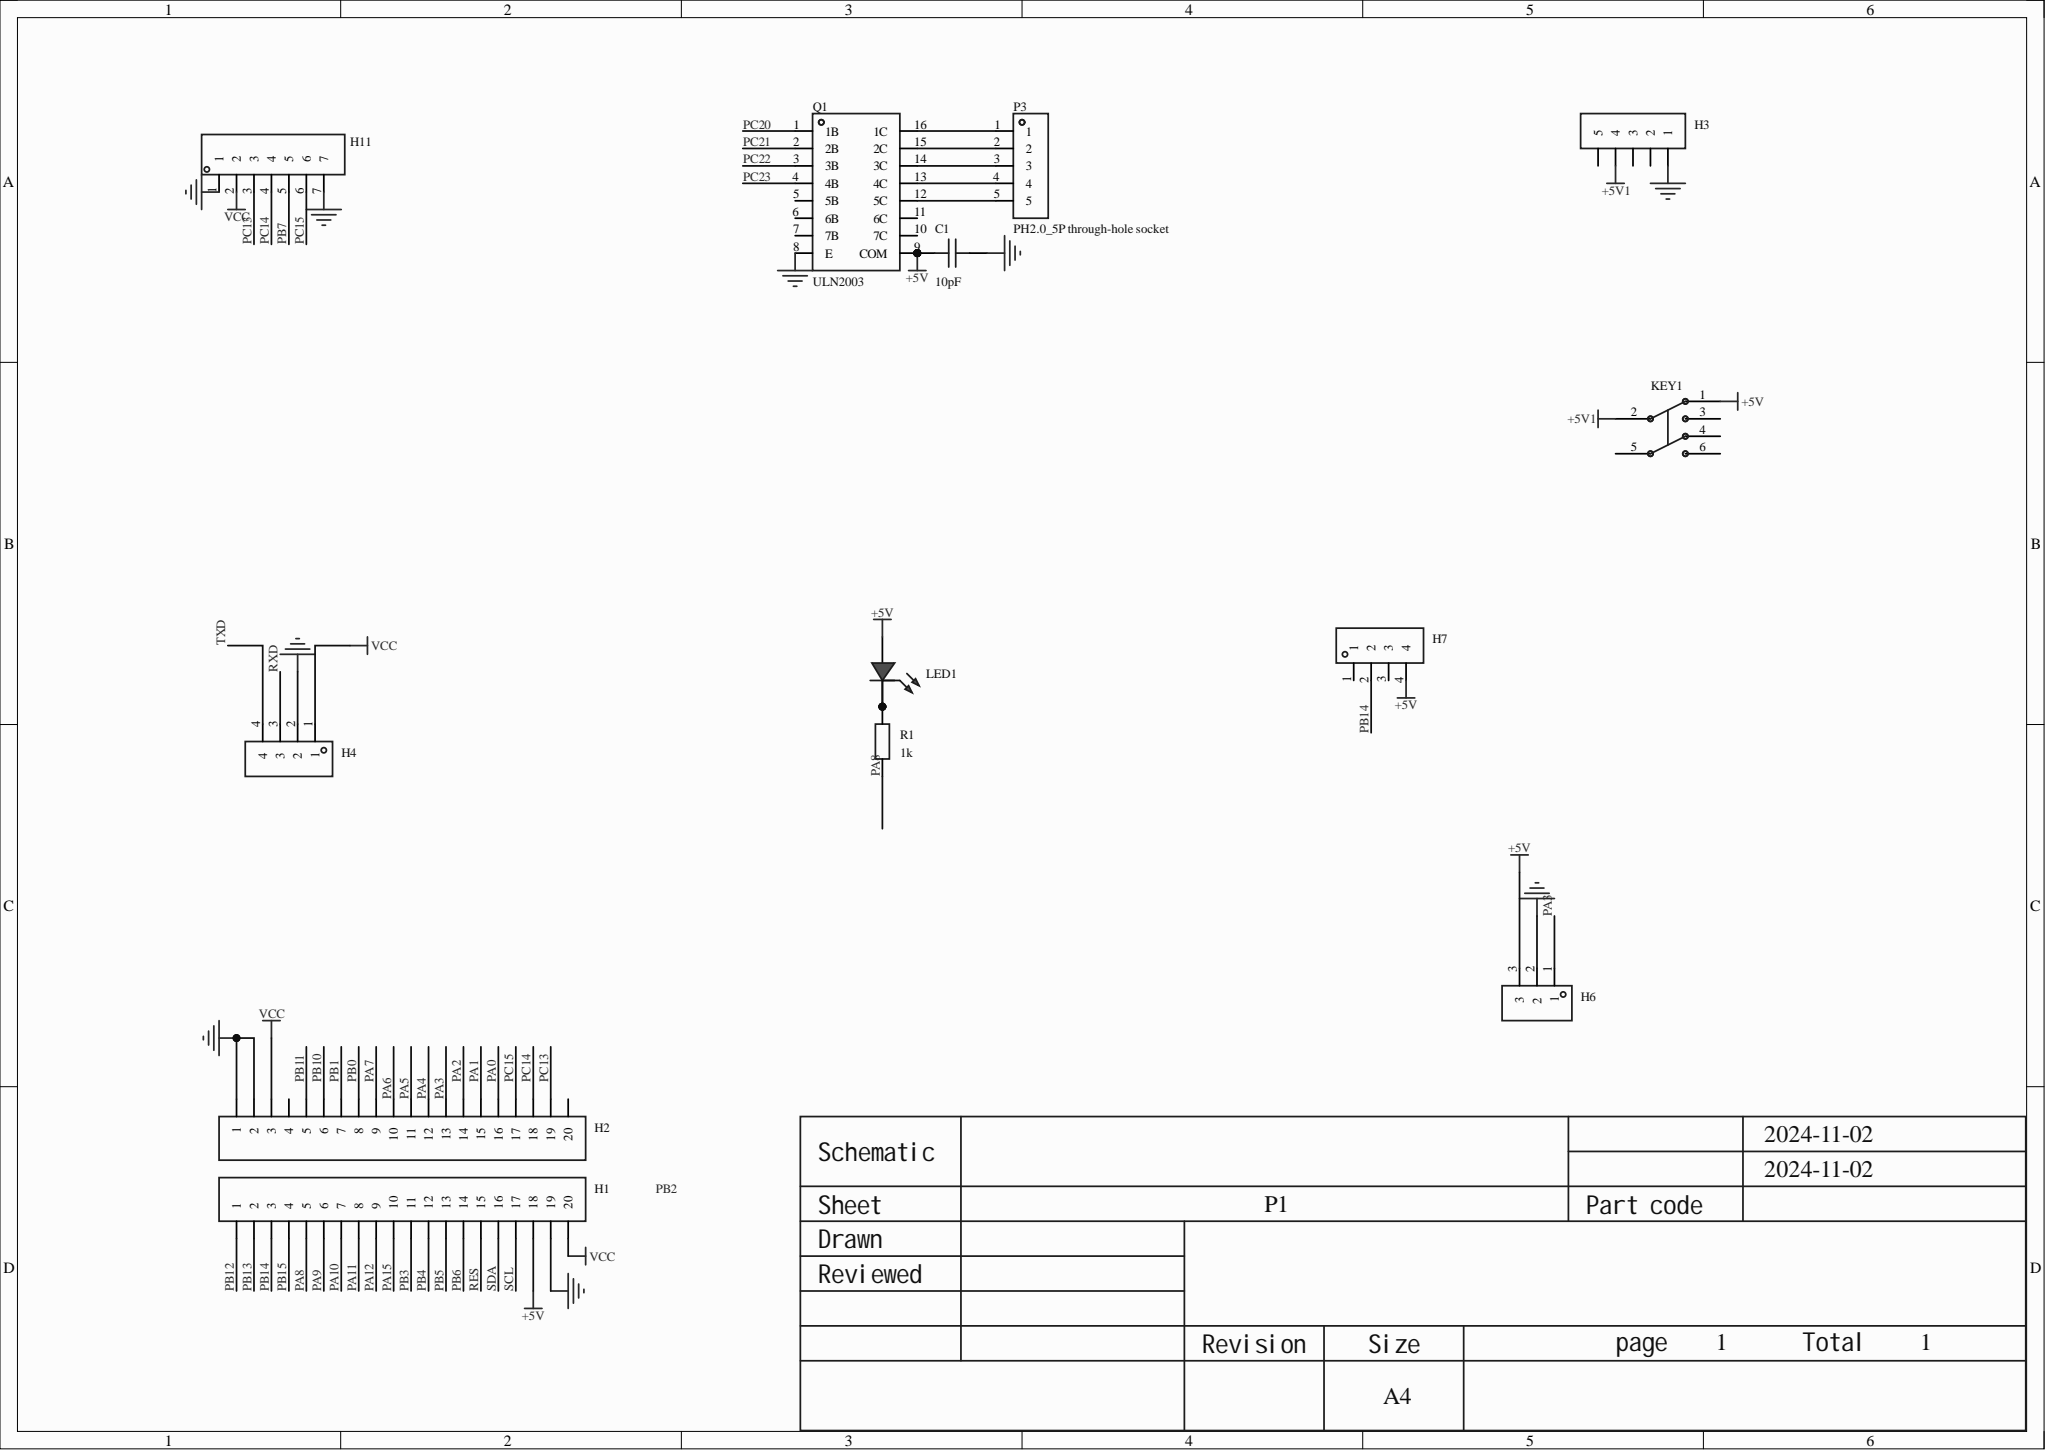Circuit board | Altium Designer | 13 parts | 16 nets
Bill of materials:
Comment,Description,Designator,Footprint,LibRef,Quantity
"10pF","容值:10pF;精度:±5%;额定电压:3kV;温度系数:SL;","C1","CAP-TH_L5.5-W6.0-P7.50-D0.6","CC45SL3FD100JYGNA","1"
"","","H1, H2","HDR-TH_20P-P2.54-V-F","HDR-F_2.54_1x20P","2"
"","","H3","HDR-TH_5P-P2.54-V-F","HDR-F_2.54_1x5P","1"
"","","H4, H7","HDR-TH_4P-P2.54-V-F","HDR-F_2.54_1x4P","2"
"","","H6","HDR-TH_3P-P2.54-V-F","HDR-F_2.54_1x3P","1"
"","","H11","HDR-TH_7P-P2.54-V-F","HDR-F_2.54_1x7P","1"
"Non-self-locking switch 8.5×8.5 silent","6脚，8.5×8.5","KEY1","SW-TH_6P-L8.5-W8.5-P2.54","无自锁开关 8.5×8.5 无声","1"
"","","LED1","LED_TH-_5mm","LED_TH-R_5mm","1"
"PH2.0_5P through-hole socket","","P3","CONN-TH_5P-P2.00-PH5A","PH2.0_5P直插插座","1"
"ULN2003","","Q1","DIP-16_L19.8-W6.5-P2.54-LS7.6-BL","ULN2003_C557872","1"
"1k","","R1","Res_1/4W","Res_AXIAL-1/4W","1"
Netlist (Protel format):
[
C1
CAP-TH_L5.5-W6.0-P7.50-D0.6
10pF



]
[
H1
HDR-TH_20P-P2.54-V-F




]
[
H2
HDR-TH_20P-P2.54-V-F




]
[
H3
HDR-TH_5P-P2.54-V-F




]
[
H4
HDR-TH_4P-P2.54-V-F




]
[
H6
HDR-TH_3P-P2.54-V-F




]
[
H7
HDR-TH_4P-P2.54-V-F




]
[
H11
HDR-TH_7P-P2.54-V-F




]
[
KEY1
SW-TH_6P-L8.5-W8.5-P2.54
Non-self-locking switch 8.5×8.5 silent



]
[
LED1
LED_TH-_5mm




]
[
P3
CONN-TH_5P-P2.00-PH5A
PH2.0_5P through-hole socket



]
[
Q1
DIP-16_L19.8-W6.5-P2.54-LS7.6-BL
ULN2003



]
[
R1
Res_1/4W
1k



]
(
VCC
H1-20
H2-3
H4-1
H11-2
)
(
PC15
H2-17
H11-6
)
(
PC14
H2-18
H11-4
)
(
PC13
H2-19
H11-3
)
(
PB14
H1-3
H7-2
)
(
PA8
H1-5
R1-1
)
(
PA3
H2-13
H6-1
)
(
NetP3_5
P3-5
Q1-12
)
(
NetP3_4
P3-4
Q1-13
)
(
NetP3_3
P3-3
Q1-14
)
(
NetP3_2
P3-2
Q1-15
)
(
NetP3_1
P3-1
Q1-16
)
(
NetLED1_2
LED1-2
R1-2
)
(
GND
C1-2
H1-19
H2-1
H2-2
H3-1
H4-2
H6-2
H11-1
H11-7
Q1-8
)
(
+5V1
H3-4
KEY1-2
)
(
+5V
C1-1
H1-18
H6-3
H7-4
KEY1-1
LED1-1
Q1-9
)